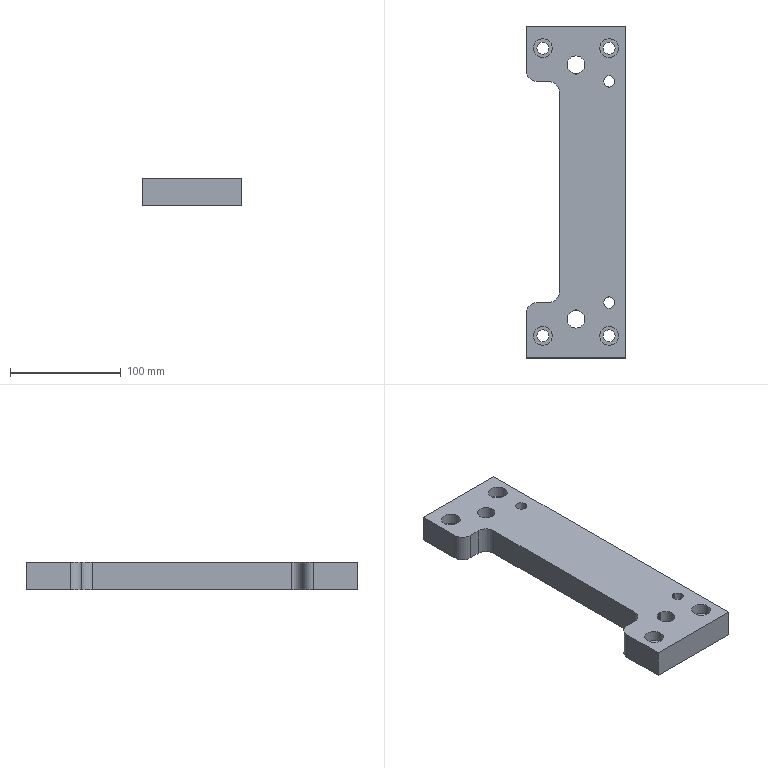Part | STEP file | YBQDJ-QD-1 | 1 solid | 46 faces | box 90 x 300 x 25 mm | volume 495978 mm3 | cylinder 28 | plane 16 | cone 2 | commonest cylinder face diameters 4 x8 1 x4 10.7 x4 17 x4 20 x4 10.01 x2